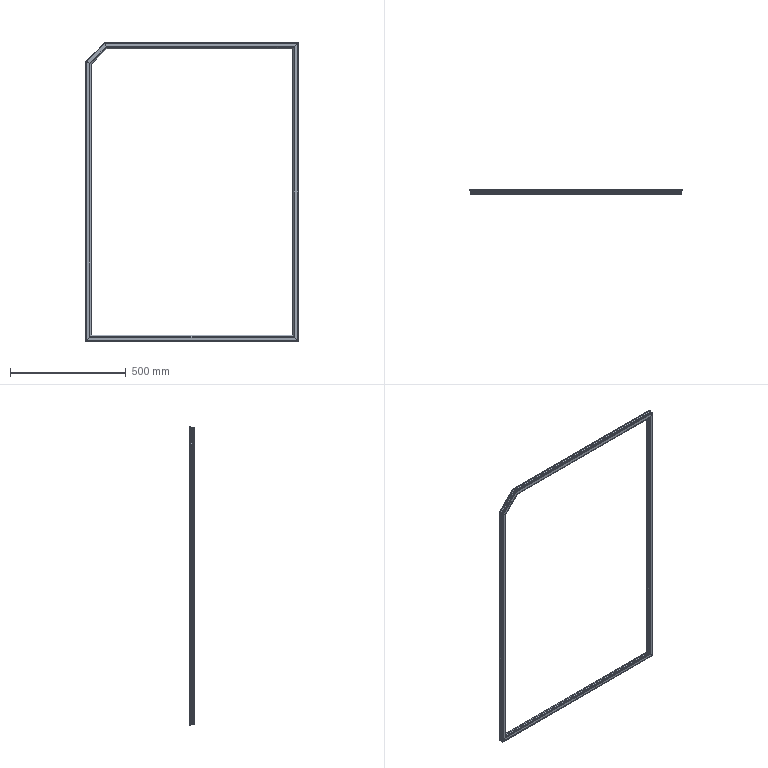Part | NX | features BREP 40 | 40 solids | 640 faces | box 921.878 x 23.5 x 1292 mm | volume 1729041 mm3 | cylinder 340 | plane 300 | commonest cylinder face diameters 2 x50 1 x40 4 x40 6 x30 1.2 x20 10 x20